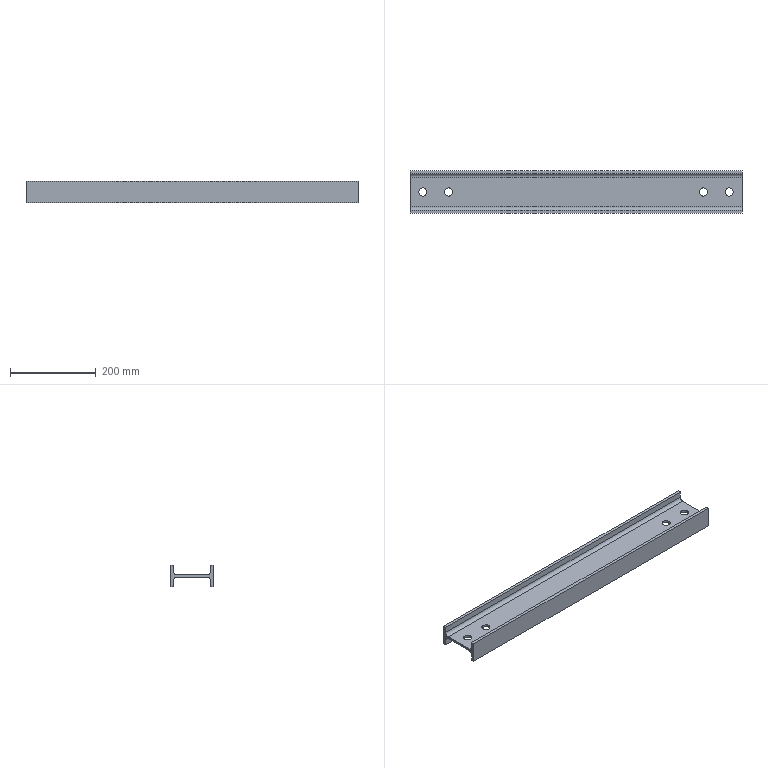Part | STEP file | 粉仓辅梁3主体_Default<As Machined> | 1 solid | 26 faces | box 775 x 100 x 50 mm | volume 912656 mm3 | plane 14 | cylinder 12 | commonest cylinder face diameters 19 x8 16 x4